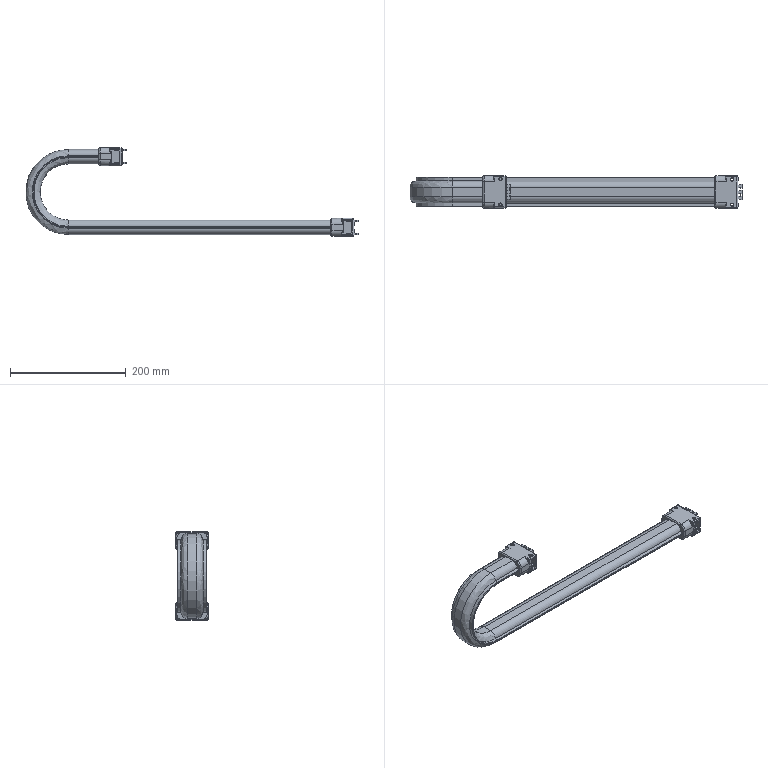Part | SolidWorks | features BaseBody 3 | 3 solids | 511 faces | box 573.5 x 56 x 153.4 mm | volume 269954 mm3 | plane 256 | cylinder 186 | cone 37 | spline 32 | commonest cylinder face diameters 4 x40 4.5 x32 6 x32 7 x32 5 x8 17 x8